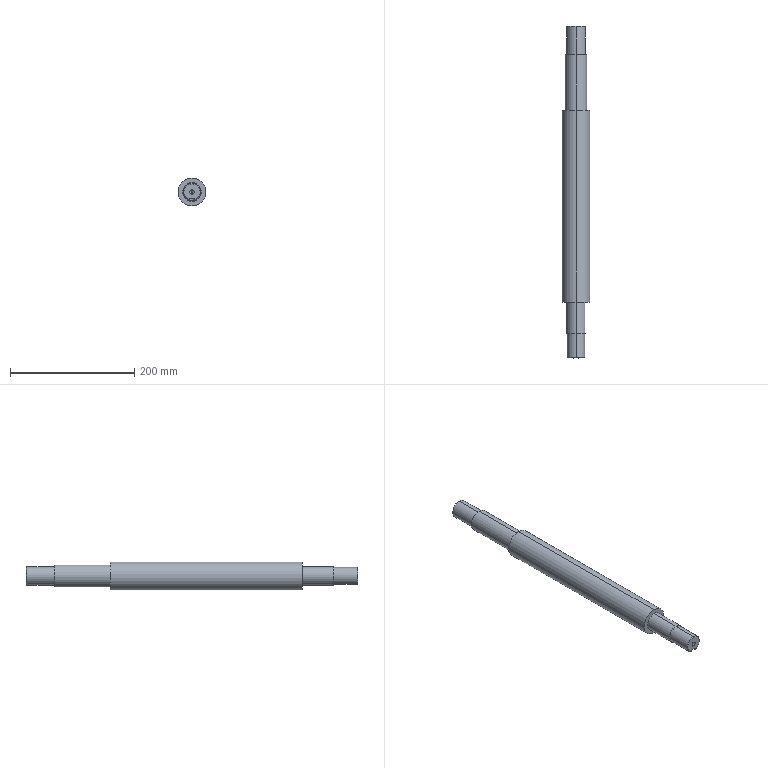Part | SolidWorks | features 3DProfileFeature 1, Chamfer 1, Cut 1, HoleWzd 1, Revolution 1 | 1 solid | 28 faces | box 45 x 535 x 45 mm | volume 668255 mm3 | cylinder 13 | plane 9 | cone 6 | commonest cylinder face diameters 30 x4 7 x2 28 x2 35 x2 45 x2 8 x1
STEP:
#1=CARTESIAN_POINT('',(0.,25.,3.5));
#2=VERTEX_POINT('',#1);
#3=CARTESIAN_POINT('',(0.,25.,-3.5));
#4=VERTEX_POINT('',#3);
#5=CARTESIAN_POINT('',(0.,25.,0.));
#6=DIRECTION('',(0.,-1.,0.));
#7=DIRECTION('',(0.,0.,-1.));
#8=AXIS2_PLACEMENT_3D('',#5,#6,#7);
#9=CIRCLE('',#8,3.5);
#10=EDGE_CURVE('',#2,#4,#9,.T.);
#11=ORIENTED_EDGE('',*,*,#10,.F.);
#12=CARTESIAN_POINT('',(0.,0.,3.5));
#13=VERTEX_POINT('',#12);
#14=CARTESIAN_POINT('',(0.,0.,3.5));
#15=DIRECTION('',(0.,-1.,0.));
#16=VECTOR('',#15,1000.);
#17=LINE('',#14,#16);
#18=EDGE_CURVE('',#2,#13,#17,.T.);
#19=ORIENTED_EDGE('',*,*,#18,.T.);
#20=CARTESIAN_POINT('',(0.,0.,-3.5));
#21=VERTEX_POINT('',#20);
#22=CARTESIAN_POINT('',(0.,0.,0.));
#23=DIRECTION('',(0.,-1.,0.));
#24=DIRECTION('',(0.,0.,-1.));
#25=AXIS2_PLACEMENT_3D('',#22,#23,#24);
#26=CIRCLE('',#25,3.5);
#27=EDGE_CURVE('',#13,#21,#26,.T.);
#28=ORIENTED_EDGE('',*,*,#27,.T.);
#29=CARTESIAN_POINT('',(0.,0.,-3.5));
#30=DIRECTION('',(0.,-1.,0.));
#31=VECTOR('',#30,1000.);
#32=LINE('',#29,#31);
#33=EDGE_CURVE('',#4,#21,#32,.T.);
#34=ORIENTED_EDGE('',*,*,#33,.F.);
#35=EDGE_LOOP('',(#11,#19,#28,#34));
#36=FACE_OUTER_BOUND('',#35,.T.);
#37=CARTESIAN_POINT('',(0.,0.,0.));
#38=DIRECTION('',(0.,-1.,0.));
#39=DIRECTION('',(0.,0.,-1.));
#40=AXIS2_PLACEMENT_3D('',#37,#38,#39);
#41=CYLINDRICAL_SURFACE('',#40,3.5);
#42=ADVANCED_FACE('',(#36),#41,.F.);
#43=CARTESIAN_POINT('',(0.,27.103,0.));
#44=VERTEX_POINT('',#43);
#45=CARTESIAN_POINT('',(0.,25.,-3.5));
#46=DIRECTION('',(0.,-0.515,-0.8572));
#47=VECTOR('',#46,1000.);
#48=LINE('',#45,#47);
#49=EDGE_CURVE('',#44,#4,#48,.T.);
#50=ORIENTED_EDGE('',*,*,#49,.F.);
#51=CARTESIAN_POINT('',(0.,25.,3.5));
#52=DIRECTION('',(0.,-0.515,0.8572));
#53=VECTOR('',#52,1000.);
#54=LINE('',#51,#53);
#55=EDGE_CURVE('',#44,#2,#54,.T.);
#56=ORIENTED_EDGE('',*,*,#55,.T.);
#57=ORIENTED_EDGE('',*,*,#10,.T.);
#58=EDGE_LOOP('',(#50,#56,#57));
#59=FACE_OUTER_BOUND('',#58,.T.);
#60=CARTESIAN_POINT('',(0.,25.,0.));
#61=DIRECTION('',(0.,-1.,0.));
#62=DIRECTION('',(0.,0.,-1.));
#63=AXIS2_PLACEMENT_3D('',#60,#61,#62);
#64=CONICAL_SURFACE('',#63,3.5,1.03);
#65=ADVANCED_FACE('',(#59),#64,.F.);
#66=CARTESIAN_POINT('',(0.,535.,14.));
#67=VERTEX_POINT('',#66);
#68=CARTESIAN_POINT('',(0.,535.,-14.));
#69=VERTEX_POINT('',#68);
#70=CARTESIAN_POINT('',(0.,535.,0.));
#71=DIRECTION('',(0.,1.,0.));
#72=DIRECTION('',(0.,0.,-1.));
#73=AXIS2_PLACEMENT_3D('',#70,#71,#72);
#74=CIRCLE('',#73,14.);
#75=EDGE_CURVE('',#67,#69,#74,.T.);
#76=ORIENTED_EDGE('',*,*,#75,.F.);
#77=CARTESIAN_POINT('',(0.,534.,15.));
#78=VERTEX_POINT('',#77);
#79=CARTESIAN_POINT('',(0.,535.,14.));
#80=DIRECTION('',(0.,-0.7071,0.7071));
#81=VECTOR('',#80,1000.);
#82=LINE('',#79,#81);
#83=EDGE_CURVE('',#67,#78,#82,.T.);
#84=ORIENTED_EDGE('',*,*,#83,.T.);
#85=CARTESIAN_POINT('',(0.,534.,-15.));
#86=VERTEX_POINT('',#85);
#87=CARTESIAN_POINT('',(0.,534.,0.));
#88=DIRECTION('',(0.,-1.,0.));
#89=DIRECTION('',(0.,0.,-1.));
#90=AXIS2_PLACEMENT_3D('',#87,#88,#89);
#91=CIRCLE('',#90,15.);
#92=EDGE_CURVE('',#86,#78,#91,.T.);
#93=ORIENTED_EDGE('',*,*,#92,.F.);
#94=CARTESIAN_POINT('',(0.,535.,-14.));
#95=DIRECTION('',(0.,-0.7071,-0.7071));
#96=VECTOR('',#95,1000.);
#97=LINE('',#94,#96);
#98=EDGE_CURVE('',#69,#86,#97,.T.);
#99=ORIENTED_EDGE('',*,*,#98,.F.);
#100=EDGE_LOOP('',(#76,#84,#93,#99));
#101=FACE_OUTER_BOUND('',#100,.T.);
#102=CARTESIAN_POINT('',(0.,535.,0.));
#103=DIRECTION('',(0.,-1.,0.));
#104=DIRECTION('',(0.,0.,-1.));
#105=AXIS2_PLACEMENT_3D('',#102,#103,#104);
#106=CONICAL_SURFACE('',#105,14.,0.7854);
#107=ADVANCED_FACE('',(#101),#106,.T.);
#108=CARTESIAN_POINT('',(0.,0.,13.));
#109=VERTEX_POINT('',#108);
#110=CARTESIAN_POINT('',(-4.,0.,-12.369));
#111=VERTEX_POINT('',#110);
#112=CARTESIAN_POINT('',(0.,0.,0.));
#113=DIRECTION('',(0.,-1.,0.));
#114=DIRECTION('',(0.,0.,1.));
#115=AXIS2_PLACEMENT_3D('',#112,#113,#114);
#116=CIRCLE('',#115,13.);
#117=EDGE_CURVE('',#109,#111,#116,.T.);
#118=ORIENTED_EDGE('',*,*,#117,.F.);
#119=CARTESIAN_POINT('',(0.,1.,14.));
#120=VERTEX_POINT('',#119);
#121=CARTESIAN_POINT('',(0.,1.,14.));
#122=DIRECTION('',(0.,0.7071,0.7071));
#123=VECTOR('',#122,1000.);
#124=LINE('',#121,#123);
#125=EDGE_CURVE('',#109,#120,#124,.T.);
#126=ORIENTED_EDGE('',*,*,#125,.T.);
#127=CARTESIAN_POINT('',(-4.,1.,-13.416));
#128=VERTEX_POINT('',#127);
#129=CARTESIAN_POINT('',(0.,1.,0.));
#130=DIRECTION('',(0.,1.,0.));
#131=DIRECTION('',(0.,0.,1.));
#132=AXIS2_PLACEMENT_3D('',#129,#130,#131);
#133=CIRCLE('',#132,14.);
#134=EDGE_CURVE('',#128,#120,#133,.T.);
#135=ORIENTED_EDGE('',*,*,#134,.F.);
#136=CARTESIAN_POINT('',(-4.,0.,-12.369));
#137=CARTESIAN_POINT('',(-4.,0.3327,-12.719));
#138=CARTESIAN_POINT('',(-4.,0.6661,-13.068));
#139=CARTESIAN_POINT('',(-4.,1.,-13.416));
#140=B_SPLINE_CURVE_WITH_KNOTS('',3,(#136,#137,#138,#139),.UNSPECIFIED.,.F.,.F.,(4,4),(0.006639,0.008087),.UNSPECIFIED.);
#141=EDGE_CURVE('',#111,#128,#140,.T.);
#142=ORIENTED_EDGE('',*,*,#141,.F.);
#143=EDGE_LOOP('',(#118,#126,#135,#142));
#144=FACE_OUTER_BOUND('',#143,.T.);
#145=CARTESIAN_POINT('',(0.,1.,0.));
#146=DIRECTION('',(0.,1.,0.));
#147=DIRECTION('',(0.,0.,1.));
#148=AXIS2_PLACEMENT_3D('',#145,#146,#147);
#149=CONICAL_SURFACE('',#148,14.,0.7854);
#150=ADVANCED_FACE('',(#144),#149,.T.);
#151=CARTESIAN_POINT('',(0.,489.,15.));
#152=VERTEX_POINT('',#151);
#153=CARTESIAN_POINT('',(0.,489.,-15.));
#154=VERTEX_POINT('',#153);
#155=CARTESIAN_POINT('',(0.,489.,0.));
#156=DIRECTION('',(0.,1.,0.));
#157=DIRECTION('',(0.,0.,1.));
#158=AXIS2_PLACEMENT_3D('',#155,#156,#157);
#159=CIRCLE('',#158,15.);
#160=EDGE_CURVE('',#152,#154,#159,.T.);
#161=ORIENTED_EDGE('',*,*,#160,.T.);
#162=CARTESIAN_POINT('',(0.,535.,-15.));
#163=DIRECTION('',(0.,1.,0.));
#164=VECTOR('',#163,1000.);
#165=LINE('',#162,#164);
#166=EDGE_CURVE('',#154,#86,#165,.T.);
#167=ORIENTED_EDGE('',*,*,#166,.T.);
#168=ORIENTED_EDGE('',*,*,#92,.T.);
#169=CARTESIAN_POINT('',(0.,535.,15.));
#170=DIRECTION('',(0.,1.,0.));
#171=VECTOR('',#170,1000.);
#172=LINE('',#169,#171);
#173=EDGE_CURVE('',#152,#78,#172,.T.);
#174=ORIENTED_EDGE('',*,*,#173,.F.);
#175=EDGE_LOOP('',(#161,#167,#168,#174));
#176=FACE_OUTER_BOUND('',#175,.T.);
#177=CARTESIAN_POINT('',(0.,535.,0.));
#178=DIRECTION('',(0.,1.,0.));
#179=DIRECTION('',(0.,0.,1.));
#180=AXIS2_PLACEMENT_3D('',#177,#178,#179);
#181=CYLINDRICAL_SURFACE('',#180,15.);
#182=ADVANCED_FACE('',(#176),#181,.T.);
#183=CARTESIAN_POINT('',(0.,399.,17.5));
#184=VERTEX_POINT('',#183);
#185=CARTESIAN_POINT('',(0.,399.,-17.5));
#186=VERTEX_POINT('',#185);
#187=CARTESIAN_POINT('',(0.,399.,0.));
#188=DIRECTION('',(0.,1.,0.));
#189=DIRECTION('',(0.,0.,1.));
#190=AXIS2_PLACEMENT_3D('',#187,#188,#189);
#191=CIRCLE('',#190,17.5);
#192=EDGE_CURVE('',#184,#186,#191,.T.);
#193=ORIENTED_EDGE('',*,*,#192,.T.);
#194=CARTESIAN_POINT('',(0.,489.,-17.5));
#195=VERTEX_POINT('',#194);
#196=CARTESIAN_POINT('',(0.,535.,-17.5));
#197=DIRECTION('',(0.,1.,0.));
#198=VECTOR('',#197,1000.);
#199=LINE('',#196,#198);
#200=EDGE_CURVE('',#186,#195,#199,.T.);
#201=ORIENTED_EDGE('',*,*,#200,.T.);
#202=CARTESIAN_POINT('',(0.,489.,17.5));
#203=VERTEX_POINT('',#202);
#204=CARTESIAN_POINT('',(0.,489.,0.));
#205=DIRECTION('',(0.,1.,0.));
#206=DIRECTION('',(0.,0.,1.));
#207=AXIS2_PLACEMENT_3D('',#204,#205,#206);
#208=CIRCLE('',#207,17.5);
#209=EDGE_CURVE('',#203,#195,#208,.T.);
#210=ORIENTED_EDGE('',*,*,#209,.F.);
#211=CARTESIAN_POINT('',(0.,535.,17.5));
#212=DIRECTION('',(0.,1.,0.));
#213=VECTOR('',#212,1000.);
#214=LINE('',#211,#213);
#215=EDGE_CURVE('',#184,#203,#214,.T.);
#216=ORIENTED_EDGE('',*,*,#215,.F.);
#217=EDGE_LOOP('',(#193,#201,#210,#216));
#218=FACE_OUTER_BOUND('',#217,.T.);
#219=CARTESIAN_POINT('',(0.,535.,0.));
#220=DIRECTION('',(0.,1.,0.));
#221=DIRECTION('',(0.,0.,1.));
#222=AXIS2_PLACEMENT_3D('',#219,#220,#221);
#223=CYLINDRICAL_SURFACE('',#222,17.5);
#224=ADVANCED_FACE('',(#218),#223,.T.);
#225=CARTESIAN_POINT('',(0.,90.,22.5));
#226=VERTEX_POINT('',#225);
#227=CARTESIAN_POINT('',(0.,90.,-22.5));
#228=VERTEX_POINT('',#227);
#229=CARTESIAN_POINT('',(0.,90.,0.));
#230=DIRECTION('',(0.,1.,0.));
#231=DIRECTION('',(0.,0.,1.));
#232=AXIS2_PLACEMENT_3D('',#229,#230,#231);
#233=CIRCLE('',#232,22.5);
#234=EDGE_CURVE('',#226,#228,#233,.T.);
#235=ORIENTED_EDGE('',*,*,#234,.T.);
#236=CARTESIAN_POINT('',(0.,399.,-22.5));
#237=VERTEX_POINT('',#236);
#238=CARTESIAN_POINT('',(0.,535.,-22.5));
#239=DIRECTION('',(0.,1.,0.));
#240=VECTOR('',#239,1000.);
#241=LINE('',#238,#240);
#242=EDGE_CURVE('',#228,#237,#241,.T.);
#243=ORIENTED_EDGE('',*,*,#242,.T.);
#244=CARTESIAN_POINT('',(0.,399.,22.5));
#245=VERTEX_POINT('',#244);
#246=CARTESIAN_POINT('',(0.,399.,0.));
#247=DIRECTION('',(0.,1.,0.));
#248=DIRECTION('',(0.,0.,1.));
#249=AXIS2_PLACEMENT_3D('',#246,#247,#248);
#250=CIRCLE('',#249,22.5);
#251=EDGE_CURVE('',#245,#237,#250,.T.);
#252=ORIENTED_EDGE('',*,*,#251,.F.);
#253=CARTESIAN_POINT('',(0.,535.,22.5));
#254=DIRECTION('',(0.,1.,0.));
#255=VECTOR('',#254,1000.);
#256=LINE('',#253,#255);
#257=EDGE_CURVE('',#226,#245,#256,.T.);
#258=ORIENTED_EDGE('',*,*,#257,.F.);
#259=EDGE_LOOP('',(#235,#243,#252,#258));
#260=FACE_OUTER_BOUND('',#259,.T.);
#261=CARTESIAN_POINT('',(0.,535.,0.));
#262=DIRECTION('',(0.,1.,0.));
#263=DIRECTION('',(0.,0.,1.));
#264=AXIS2_PLACEMENT_3D('',#261,#262,#263);
#265=CYLINDRICAL_SURFACE('',#264,22.5);
#266=ADVANCED_FACE('',(#260),#265,.T.);
#267=CARTESIAN_POINT('',(0.,40.,15.));
#268=VERTEX_POINT('',#267);
#269=CARTESIAN_POINT('',(0.,40.,-15.));
#270=VERTEX_POINT('',#269);
#271=CARTESIAN_POINT('',(0.,40.,0.));
#272=DIRECTION('',(0.,1.,0.));
#273=DIRECTION('',(0.,0.,1.));
#274=AXIS2_PLACEMENT_3D('',#271,#272,#273);
#275=CIRCLE('',#274,15.);
#276=EDGE_CURVE('',#268,#270,#275,.T.);
#277=ORIENTED_EDGE('',*,*,#276,.T.);
#278=CARTESIAN_POINT('',(0.,90.,-15.));
#279=VERTEX_POINT('',#278);
#280=CARTESIAN_POINT('',(0.,535.,-15.));
#281=DIRECTION('',(0.,1.,0.));
#282=VECTOR('',#281,1000.);
#283=LINE('',#280,#282);
#284=EDGE_CURVE('',#270,#279,#283,.T.);
#285=ORIENTED_EDGE('',*,*,#284,.T.);
#286=CARTESIAN_POINT('',(0.,90.,15.));
#287=VERTEX_POINT('',#286);
#288=CARTESIAN_POINT('',(0.,90.,0.));
#289=DIRECTION('',(0.,1.,0.));
#290=DIRECTION('',(0.,0.,1.));
#291=AXIS2_PLACEMENT_3D('',#288,#289,#290);
#292=CIRCLE('',#291,15.);
#293=EDGE_CURVE('',#287,#279,#292,.T.);
#294=ORIENTED_EDGE('',*,*,#293,.F.);
#295=CARTESIAN_POINT('',(0.,535.,15.));
#296=DIRECTION('',(0.,1.,0.));
#297=VECTOR('',#296,1000.);
#298=LINE('',#295,#297);
#299=EDGE_CURVE('',#268,#287,#298,.T.);
#300=ORIENTED_EDGE('',*,*,#299,.F.);
#301=EDGE_LOOP('',(#277,#285,#294,#300));
#302=FACE_OUTER_BOUND('',#301,.T.);
#303=CARTESIAN_POINT('',(0.,535.,0.));
#304=DIRECTION('',(0.,1.,0.));
#305=DIRECTION('',(0.,0.,1.));
#306=AXIS2_PLACEMENT_3D('',#303,#304,#305);
#307=CYLINDRICAL_SURFACE('',#306,15.);
#308=ADVANCED_FACE('',(#302),#307,.T.);
#309=ORIENTED_EDGE('',*,*,#134,.T.);
#310=CARTESIAN_POINT('',(0.,40.,14.));
#311=VERTEX_POINT('',#310);
#312=CARTESIAN_POINT('',(0.,535.,14.));
#313=DIRECTION('',(0.,1.,0.));
#314=VECTOR('',#313,1000.);
#315=LINE('',#312,#314);
#316=EDGE_CURVE('',#120,#311,#315,.T.);
#317=ORIENTED_EDGE('',*,*,#316,.T.);
#318=CARTESIAN_POINT('',(0.,40.,-14.));
#319=VERTEX_POINT('',#318);
#320=CARTESIAN_POINT('',(0.,40.,0.));
#321=DIRECTION('',(0.,1.,0.));
#322=DIRECTION('',(0.,0.,1.));
#323=AXIS2_PLACEMENT_3D('',#320,#321,#322);
#324=CIRCLE('',#323,14.);
#325=EDGE_CURVE('',#319,#311,#324,.T.);
#326=ORIENTED_EDGE('',*,*,#325,.F.);
#327=CARTESIAN_POINT('',(-4.,36.,-13.416));
#328=VERTEX_POINT('',#327);
#329=CARTESIAN_POINT('',(0.,40.,-14.));
#330=CARTESIAN_POINT('',(-0.2622,40.,-14.));
#331=CARTESIAN_POINT('',(-0.5286,39.974,-13.992));
#332=CARTESIAN_POINT('',(-1.042,39.871,-13.964));
#333=CARTESIAN_POINT('',(-1.292,39.795,-13.942));
#334=CARTESIAN_POINT('',(-1.778,39.593,-13.889));
#335=CARTESIAN_POINT('',(-2.009,39.468,-13.857));
#336=CARTESIAN_POINT('',(-2.441,39.18,-13.787));
#337=CARTESIAN_POINT('',(-2.644,39.013,-13.749));
#338=CARTESIAN_POINT('',(-3.013,38.643,-13.673));
#339=CARTESIAN_POINT('',(-3.178,38.443,-13.635));
#340=CARTESIAN_POINT('',(-3.467,38.011,-13.565));
#341=CARTESIAN_POINT('',(-3.593,37.778,-13.532));
#342=CARTESIAN_POINT('',(-3.793,37.296,-13.477));
#343=CARTESIAN_POINT('',(-3.87,37.047,-13.455));
#344=CARTESIAN_POINT('',(-3.973,36.531,-13.424));
#345=CARTESIAN_POINT('',(-4.,36.266,-13.416));
#346=CARTESIAN_POINT('',(-4.,36.,-13.416));
#347=B_SPLINE_CURVE_WITH_KNOTS('',3,(#329,#330,#331,#332,#333,#334,#335,#336,#337,#338,#339,#340,#341,#342,#343,#344,#345,#346),.UNSPECIFIED.,.F.,.F.,(4,2,2,2,2,2,2,2,4),(0.006287,0.007072,0.007857,0.008642,0.009427,0.01021,0.011,0.01178,0.01257),.UNSPECIFIED.);
#348=EDGE_CURVE('',#319,#328,#347,.T.);
#349=ORIENTED_EDGE('',*,*,#348,.T.);
#350=CARTESIAN_POINT('',(-4.,535.,-13.416));
#351=DIRECTION('',(0.,-1.,0.));
#352=VECTOR('',#351,1000.);
#353=LINE('',#350,#352);
#354=EDGE_CURVE('',#328,#128,#353,.T.);
#355=ORIENTED_EDGE('',*,*,#354,.T.);
#356=EDGE_LOOP('',(#309,#317,#326,#349,#355));
#357=FACE_OUTER_BOUND('',#356,.T.);
#358=CARTESIAN_POINT('',(0.,535.,0.));
#359=DIRECTION('',(0.,1.,0.));
#360=DIRECTION('',(0.,0.,1.));
#361=AXIS2_PLACEMENT_3D('',#358,#359,#360);
#362=CYLINDRICAL_SURFACE('',#361,14.);
#363=ADVANCED_FACE('',(#357),#362,.T.);
#364=CARTESIAN_POINT('',(0.,0.,0.));
#365=DIRECTION('',(0.,-1.,0.));
#366=DIRECTION('',(0.,0.,-1.));
#367=AXIS2_PLACEMENT_3D('',#364,#365,#366);
#368=CIRCLE('',#367,3.5);
#369=EDGE_CURVE('',#21,#13,#368,.T.);
#370=ORIENTED_EDGE('',*,*,#369,.F.);
#371=ORIENTED_EDGE('',*,*,#27,.F.);
#372=EDGE_LOOP('',(#370,#371));
#373=FACE_BOUND('',#372,.T.);
#374=CARTESIAN_POINT('',(-4.,0.,-10.));
#375=VERTEX_POINT('',#374);
#376=CARTESIAN_POINT('',(4.,0.,-10.));
#377=VERTEX_POINT('',#376);
#378=CARTESIAN_POINT('',(0.,0.,-10.));
#379=DIRECTION('',(1.,0.,0.));
#380=VECTOR('',#379,1000.);
#381=LINE('',#378,#380);
#382=EDGE_CURVE('',#375,#377,#381,.T.);
#383=ORIENTED_EDGE('',*,*,#382,.T.);
#384=CARTESIAN_POINT('',(4.,0.,-12.369));
#385=VERTEX_POINT('',#384);
#386=CARTESIAN_POINT('',(4.,0.,-15.));
#387=DIRECTION('',(0.,0.,1.));
#388=VECTOR('',#387,1000.);
#389=LINE('',#386,#388);
#390=EDGE_CURVE('',#385,#377,#389,.T.);
#391=ORIENTED_EDGE('',*,*,#390,.F.);
#392=CARTESIAN_POINT('',(0.,0.,0.));
#393=DIRECTION('',(0.,-1.,0.));
#394=DIRECTION('',(0.,0.,1.));
#395=AXIS2_PLACEMENT_3D('',#392,#393,#394);
#396=CIRCLE('',#395,13.);
#397=EDGE_CURVE('',#385,#109,#396,.T.);
#398=ORIENTED_EDGE('',*,*,#397,.T.);
#399=ORIENTED_EDGE('',*,*,#117,.T.);
#400=CARTESIAN_POINT('',(-4.,0.,-15.));
#401=DIRECTION('',(0.,0.,1.));
#402=VECTOR('',#401,1000.);
#403=LINE('',#400,#402);
#404=EDGE_CURVE('',#111,#375,#403,.T.);
#405=ORIENTED_EDGE('',*,*,#404,.T.);
#406=EDGE_LOOP('',(#383,#391,#398,#399,#405));
#407=FACE_OUTER_BOUND('',#406,.T.);
#408=CARTESIAN_POINT('',(0.,0.,0.));
#409=DIRECTION('',(0.,1.,0.));
#410=DIRECTION('',(0.,0.,1.));
#411=AXIS2_PLACEMENT_3D('',#408,#409,#410);
#412=PLANE('',#411);
#413=ADVANCED_FACE('',(#373,#407),#412,.F.);
#414=ORIENTED_EDGE('',*,*,#316,.F.);
#415=CARTESIAN_POINT('',(4.,1.,-13.416));
#416=VERTEX_POINT('',#415);
#417=CARTESIAN_POINT('',(0.,1.,0.));
#418=DIRECTION('',(0.,1.,0.));
#419=DIRECTION('',(0.,0.,1.));
#420=AXIS2_PLACEMENT_3D('',#417,#418,#419);
#421=CIRCLE('',#420,14.);
#422=EDGE_CURVE('',#120,#416,#421,.T.);
#423=ORIENTED_EDGE('',*,*,#422,.T.);
#424=CARTESIAN_POINT('',(4.,36.,-13.416));
#425=VERTEX_POINT('',#424);
#426=CARTESIAN_POINT('',(4.,535.,-13.416));
#427=DIRECTION('',(0.,1.,0.));
#428=VECTOR('',#427,1000.);
#429=LINE('',#426,#428);
#430=EDGE_CURVE('',#416,#425,#429,.T.);
#431=ORIENTED_EDGE('',*,*,#430,.T.);
#432=CARTESIAN_POINT('',(4.,36.,-13.416));
#433=CARTESIAN_POINT('',(4.,36.266,-13.416));
#434=CARTESIAN_POINT('',(3.974,36.527,-13.424));
#435=CARTESIAN_POINT('',(3.871,37.04,-13.454));
#436=CARTESIAN_POINT('',(3.794,37.295,-13.477));
#437=CARTESIAN_POINT('',(3.592,37.779,-13.532));
#438=CARTESIAN_POINT('',(3.469,38.008,-13.564));
#439=CARTESIAN_POINT('',(3.179,38.442,-13.635));
#440=CARTESIAN_POINT('',(3.011,38.646,-13.674));
#441=CARTESIAN_POINT('',(2.644,39.013,-13.749));
#442=CARTESIAN_POINT('',(2.443,39.178,-13.787));
#443=CARTESIAN_POINT('',(2.006,39.471,-13.857));
#444=CARTESIAN_POINT('',(1.775,39.594,-13.889));
#445=CARTESIAN_POINT('',(1.294,39.794,-13.942));
#446=CARTESIAN_POINT('',(1.04,39.871,-13.964));
#447=CARTESIAN_POINT('',(0.5231,39.974,-13.993));
#448=CARTESIAN_POINT('',(0.2626,40.,-14.));
#449=CARTESIAN_POINT('',(0.,40.,-14.));
#450=B_SPLINE_CURVE_WITH_KNOTS('',3,(#432,#433,#434,#435,#436,#437,#438,#439,#440,#441,#442,#443,#444,#445,#446,#447,#448,#449),.UNSPECIFIED.,.F.,.F.,(4,2,2,2,2,2,2,2,4),(0.,0.0007859,0.001572,0.002358,0.003144,0.00393,0.004716,0.005502,0.006287),.UNSPECIFIED.);
#451=EDGE_CURVE('',#425,#319,#450,.T.);
#452=ORIENTED_EDGE('',*,*,#451,.T.);
#453=CARTESIAN_POINT('',(0.,40.,0.));
#454=DIRECTION('',(0.,1.,0.));
#455=DIRECTION('',(0.,0.,1.));
#456=AXIS2_PLACEMENT_3D('',#453,#454,#455);
#457=CIRCLE('',#456,14.);
#458=EDGE_CURVE('',#311,#319,#457,.T.);
#459=ORIENTED_EDGE('',*,*,#458,.F.);
#460=EDGE_LOOP('',(#414,#423,#431,#452,#459));
#461=FACE_OUTER_BOUND('',#460,.T.);
#462=CARTESIAN_POINT('',(0.,535.,0.));
#463=DIRECTION('',(0.,1.,0.));
#464=DIRECTION('',(0.,0.,1.));
#465=AXIS2_PLACEMENT_3D('',#462,#463,#464);
#466=CYLINDRICAL_SURFACE('',#465,14.);
#467=ADVANCED_FACE('',(#461),#466,.T.);
#468=ORIENTED_EDGE('',*,*,#325,.T.);
#469=ORIENTED_EDGE('',*,*,#458,.T.);
#470=EDGE_LOOP('',(#468,#469));
#471=FACE_BOUND('',#470,.T.);
#472=ORIENTED_EDGE('',*,*,#276,.F.);
#473=CARTESIAN_POINT('',(0.,40.,0.));
#474=DIRECTION('',(0.,1.,0.));
#475=DIRECTION('',(0.,0.,1.));
#476=AXIS2_PLACEMENT_3D('',#473,#474,#475);
#477=CIRCLE('',#476,15.);
#478=EDGE_CURVE('',#270,#268,#477,.T.);
#479=ORIENTED_EDGE('',*,*,#478,.F.);
#480=EDGE_LOOP('',(#472,#479));
#481=FACE_OUTER_BOUND('',#480,.T.);
#482=CARTESIAN_POINT('',(14.,40.,0.));
#483=DIRECTION('',(0.,1.,0.));
#484=DIRECTION('',(0.,0.,1.));
#485=AXIS2_PLACEMENT_3D('',#482,#483,#484);
#486=PLANE('',#485);
#487=ADVANCED_FACE('',(#471,#481),#486,.F.);
#488=ORIENTED_EDGE('',*,*,#284,.F.);
#489=ORIENTED_EDGE('',*,*,#478,.T.);
#490=ORIENTED_EDGE('',*,*,#299,.T.);
#491=CARTESIAN_POINT('',(0.,90.,0.));
#492=DIRECTION('',(0.,1.,0.));
#493=DIRECTION('',(0.,0.,1.));
#494=AXIS2_PLACEMENT_3D('',#491,#492,#493);
#495=CIRCLE('',#494,15.);
#496=EDGE_CURVE('',#279,#287,#495,.T.);
#497=ORIENTED_EDGE('',*,*,#496,.F.);
#498=EDGE_LOOP('',(#488,#489,#490,#497));
#499=FACE_OUTER_BOUND('',#498,.T.);
#500=CARTESIAN_POINT('',(0.,535.,0.));
#501=DIRECTION('',(0.,1.,0.));
#502=DIRECTION('',(0.,0.,1.));
#503=AXIS2_PLACEMENT_3D('',#500,#501,#502);
#504=CYLINDRICAL_SURFACE('',#503,15.);
#505=ADVANCED_FACE('',(#499),#504,.T.);
#506=ORIENTED_EDGE('',*,*,#234,.F.);
#507=CARTESIAN_POINT('',(0.,90.,0.));
#508=DIRECTION('',(0.,1.,0.));
#509=DIRECTION('',(0.,0.,1.));
#510=AXIS2_PLACEMENT_3D('',#507,#508,#509);
#511=CIRCLE('',#510,22.5);
#512=EDGE_CURVE('',#228,#226,#511,.T.);
#513=ORIENTED_EDGE('',*,*,#512,.F.);
#514=EDGE_LOOP('',(#506,#513));
#515=FACE_OUTER_BOUND('',#514,.T.);
#516=ORIENTED_EDGE('',*,*,#293,.T.);
#517=ORIENTED_EDGE('',*,*,#496,.T.);
#518=EDGE_LOOP('',(#516,#517));
#519=FACE_BOUND('',#518,.T.);
#520=CARTESIAN_POINT('',(15.,90.,0.));
#521=DIRECTION('',(0.,1.,0.));
#522=DIRECTION('',(0.,0.,1.));
#523=AXIS2_PLACEMENT_3D('',#520,#521,#522);
#524=PLANE('',#523);
#525=ADVANCED_FACE('',(#515,#519),#524,.F.);
#526=ORIENTED_EDGE('',*,*,#242,.F.);
#527=ORIENTED_EDGE('',*,*,#512,.T.);
#528=ORIENTED_EDGE('',*,*,#257,.T.);
#529=CARTESIAN_POINT('',(0.,399.,0.));
#530=DIRECTION('',(0.,1.,0.));
#531=DIRECTION('',(0.,0.,1.));
#532=AXIS2_PLACEMENT_3D('',#529,#530,#531);
#533=CIRCLE('',#532,22.5);
#534=EDGE_CURVE('',#237,#245,#533,.T.);
#535=ORIENTED_EDGE('',*,*,#534,.F.);
#536=EDGE_LOOP('',(#526,#527,#528,#535));
#537=FACE_OUTER_BOUND('',#536,.T.);
#538=CARTESIAN_POINT('',(0.,535.,0.));
#539=DIRECTION('',(0.,1.,0.));
#540=DIRECTION('',(0.,0.,1.));
#541=AXIS2_PLACEMENT_3D('',#538,#539,#540);
#542=CYLINDRICAL_SURFACE('',#541,22.5);
#543=ADVANCED_FACE('',(#537),#542,.T.);
#544=ORIENTED_EDGE('',*,*,#192,.F.);
#545=CARTESIAN_POINT('',(0.,399.,0.));
#546=DIRECTION('',(0.,1.,0.));
#547=DIRECTION('',(0.,0.,1.));
#548=AXIS2_PLACEMENT_3D('',#545,#546,#547);
#549=CIRCLE('',#548,17.5);
#550=EDGE_CURVE('',#186,#184,#549,.T.);
#551=ORIENTED_EDGE('',*,*,#550,.F.);
#552=EDGE_LOOP('',(#544,#551));
#553=FACE_BOUND('',#552,.T.);
#554=ORIENTED_EDGE('',*,*,#251,.T.);
#555=ORIENTED_EDGE('',*,*,#534,.T.);
#556=EDGE_LOOP('',(#554,#555));
#557=FACE_OUTER_BOUND('',#556,.T.);
#558=CARTESIAN_POINT('',(22.5,399.,0.));
#559=DIRECTION('',(0.,-1.,0.));
#560=DIRECTION('',(0.,0.,-1.));
#561=AXIS2_PLACEMENT_3D('',#558,#559,#560);
#562=PLANE('',#561);
#563=ADVANCED_FACE('',(#553,#557),#562,.F.);
#564=ORIENTED_EDGE('',*,*,#200,.F.);
#565=ORIENTED_EDGE('',*,*,#550,.T.);
#566=ORIENTED_EDGE('',*,*,#215,.T.);
#567=CARTESIAN_POINT('',(0.,489.,0.));
#568=DIRECTION('',(0.,1.,0.));
#569=DIRECTION('',(0.,0.,1.));
#570=AXIS2_PLACEMENT_3D('',#567,#568,#569);
#571=CIRCLE('',#570,17.5);
#572=EDGE_CURVE('',#195,#203,#571,.T.);
#573=ORIENTED_EDGE('',*,*,#572,.F.);
#574=EDGE_LOOP('',(#564,#565,#566,#573));
#575=FACE_OUTER_BOUND('',#574,.T.);
#576=CARTESIAN_POINT('',(0.,535.,0.));
#577=DIRECTION('',(0.,1.,0.));
#578=DIRECTION('',(0.,0.,1.));
#579=AXIS2_PLACEMENT_3D('',#576,#577,#578);
#580=CYLINDRICAL_SURFACE('',#579,17.5);
#581=ADVANCED_FACE('',(#575),#580,.T.);
#582=ORIENTED_EDGE('',*,*,#160,.F.);
#583=CARTESIAN_POINT('',(0.,489.,0.));
#584=DIRECTION('',(0.,1.,0.));
#585=DIRECTION('',(0.,0.,1.));
#586=AXIS2_PLACEMENT_3D('',#583,#584,#585);
#587=CIRCLE('',#586,15.);
#588=EDGE_CURVE('',#154,#152,#587,.T.);
#589=ORIENTED_EDGE('',*,*,#588,.F.);
#590=EDGE_LOOP('',(#582,#589));
#591=FACE_BOUND('',#590,.T.);
#592=ORIENTED_EDGE('',*,*,#209,.T.);
#593=ORIENTED_EDGE('',*,*,#572,.T.);
#594=EDGE_LOOP('',(#592,#593));
#595=FACE_OUTER_BOUND('',#594,.T.);
#596=CARTESIAN_POINT('',(17.5,489.,0.));
#597=DIRECTION('',(0.,-1.,0.));
#598=DIRECTION('',(0.,0.,-1.));
#599=AXIS2_PLACEMENT_3D('',#596,#597,#598);
#600=PLANE('',#599);
#601=ADVANCED_FACE('',(#591,#595),#600,.F.);
#602=ORIENTED_EDGE('',*,*,#166,.F.);
#603=ORIENTED_EDGE('',*,*,#588,.T.);
#604=ORIENTED_EDGE('',*,*,#173,.T.);
#605=CARTESIAN_POINT('',(0.,534.,0.));
#606=DIRECTION('',(0.,-1.,0.));
#607=DIRECTION('',(0.,0.,-1.));
#608=AXIS2_PLACEMENT_3D('',#605,#606,#607);
#609=CIRCLE('',#608,15.);
#610=EDGE_CURVE('',#78,#86,#609,.T.);
#611=ORIENTED_EDGE('',*,*,#610,.T.);
#612=EDGE_LOOP('',(#602,#603,#604,#611));
#613=FACE_OUTER_BOUND('',#612,.T.);
#614=CARTESIAN_POINT('',(0.,535.,0.));
#615=DIRECTION('',(0.,1.,0.));
#616=DIRECTION('',(0.,0.,1.));
#617=AXIS2_PLACEMENT_3D('',#614,#615,#616);
#618=CYLINDRICAL_SURFACE('',#617,15.);
#619=ADVANCED_FACE('',(#613),#618,.T.);
#620=CARTESIAN_POINT('',(0.,535.,0.));
#621=DIRECTION('',(0.,1.,0.));
#622=DIRECTION('',(0.,0.,-1.));
#623=AXIS2_PLACEMENT_3D('',#620,#621,#622);
#624=CIRCLE('',#623,14.);
#625=EDGE_CURVE('',#69,#67,#624,.T.);
#626=ORIENTED_EDGE('',*,*,#625,.T.);
#627=ORIENTED_EDGE('',*,*,#75,.T.);
#628=EDGE_LOOP('',(#626,#627));
#629=FACE_OUTER_BOUND('',#628,.T.);
#630=CARTESIAN_POINT('',(15.,535.,0.));
#631=DIRECTION('',(0.,-1.,0.));
#632=DIRECTION('',(0.,0.,-1.));
#633=AXIS2_PLACEMENT_3D('',#630,#631,#632);
#634=PLANE('',#633);
#635=ADVANCED_FACE('',(#629),#634,.F.);
#636=ORIENTED_EDGE('',*,*,#125,.F.);
#637=ORIENTED_EDGE('',*,*,#397,.F.);
#638=CARTESIAN_POINT('',(4.,1.,-13.416));
#639=CARTESIAN_POINT('',(4.,0.6661,-13.068));
#640=CARTESIAN_POINT('',(4.,0.3327,-12.719));
#641=CARTESIAN_POINT('',(4.,0.,-12.369));
#642=B_SPLINE_CURVE_WITH_KNOTS('',3,(#638,#639,#640,#641),.UNSPECIFIED.,.F.,.F.,(4,4),(0.007514,0.008962),.UNSPECIFIED.);
#643=EDGE_CURVE('',#416,#385,#642,.T.);
#644=ORIENTED_EDGE('',*,*,#643,.F.);
#645=ORIENTED_EDGE('',*,*,#422,.F.);
#646=EDGE_LOOP('',(#636,#637,#644,#645));
#647=FACE_OUTER_BOUND('',#646,.T.);
#648=CARTESIAN_POINT('',(0.,1.,0.));
#649=DIRECTION('',(0.,1.,0.));
#650=DIRECTION('',(0.,0.,1.));
#651=AXIS2_PLACEMENT_3D('',#648,#649,#650);
#652=CONICAL_SURFACE('',#651,14.,0.7854);
#653=ADVANCED_FACE('',(#647),#652,.T.);
#654=ORIENTED_EDGE('',*,*,#83,.F.);
#655=ORIENTED_EDGE('',*,*,#625,.F.);
#656=ORIENTED_EDGE('',*,*,#98,.T.);
#657=ORIENTED_EDGE('',*,*,#610,.F.);
#658=EDGE_LOOP('',(#654,#655,#656,#657));
#659=FACE_OUTER_BOUND('',#658,.T.);
#660=CARTESIAN_POINT('',(0.,535.,0.));
#661=DIRECTION('',(0.,-1.,0.));
#662=DIRECTION('',(0.,0.,-1.));
#663=AXIS2_PLACEMENT_3D('',#660,#661,#662);
#664=CONICAL_SURFACE('',#663,14.,0.7854);
#665=ADVANCED_FACE('',(#659),#664,.T.);
#666=CARTESIAN_POINT('',(-4.,36.,-10.));
#667=VERTEX_POINT('',#666);
#668=CARTESIAN_POINT('',(-4.,36.,-10.));
#669=DIRECTION('',(0.,-1.,0.));
#670=VECTOR('',#669,1000.);
#671=LINE('',#668,#670);
#672=EDGE_CURVE('',#667,#375,#671,.T.);
#673=ORIENTED_EDGE('',*,*,#672,.F.);
#674=CARTESIAN_POINT('',(4.,36.,-10.));
#675=VERTEX_POINT('',#674);
#676=CARTESIAN_POINT('',(0.,36.,-10.));
#677=DIRECTION('',(0.,0.,1.));
#678=DIRECTION('',(1.,0.,0.));
#679=AXIS2_PLACEMENT_3D('',#676,#677,#678);
#680=CIRCLE('',#679,4.);
#681=EDGE_CURVE('',#675,#667,#680,.T.);
#682=ORIENTED_EDGE('',*,*,#681,.F.);
#683=CARTESIAN_POINT('',(4.,36.,-10.));
#684=DIRECTION('',(0.,1.,0.));
#685=VECTOR('',#684,1000.);
#686=LINE('',#683,#685);
#687=EDGE_CURVE('',#377,#675,#686,.T.);
#688=ORIENTED_EDGE('',*,*,#687,.F.);
#689=ORIENTED_EDGE('',*,*,#382,.F.);
#690=EDGE_LOOP('',(#673,#682,#688,#689));
#691=FACE_OUTER_BOUND('',#690,.T.);
#692=CARTESIAN_POINT('',(0.,36.,-10.));
#693=DIRECTION('',(0.,0.,1.));
#694=DIRECTION('',(1.,0.,0.));
#695=AXIS2_PLACEMENT_3D('',#692,#693,#694);
#696=PLANE('',#695);
#697=ADVANCED_FACE('',(#691),#696,.F.);
#698=CARTESIAN_POINT('',(4.,36.,-15.));
#699=DIRECTION('',(0.,0.,1.));
#700=VECTOR('',#699,1000.);
#701=LINE('',#698,#700);
#702=EDGE_CURVE('',#425,#675,#701,.T.);
#703=ORIENTED_EDGE('',*,*,#702,.T.);
#704=ORIENTED_EDGE('',*,*,#681,.T.);
#705=CARTESIAN_POINT('',(-4.,36.,-15.));
#706=DIRECTION('',(0.,0.,1.));
#707=VECTOR('',#706,1000.);
#708=LINE('',#705,#707);
#709=EDGE_CURVE('',#328,#667,#708,.T.);
#710=ORIENTED_EDGE('',*,*,#709,.F.);
#711=ORIENTED_EDGE('',*,*,#348,.F.);
#712=ORIENTED_EDGE('',*,*,#451,.F.);
#713=EDGE_LOOP('',(#703,#704,#710,#711,#712));
#714=FACE_OUTER_BOUND('',#713,.T.);
#715=CARTESIAN_POINT('',(0.,36.,-15.));
#716=DIRECTION('',(0.,0.,1.));
#717=DIRECTION('',(1.,0.,0.));
#718=AXIS2_PLACEMENT_3D('',#715,#716,#717);
#719=CYLINDRICAL_SURFACE('',#718,4.);
#720=ADVANCED_FACE('',(#714),#719,.F.);
#721=ORIENTED_EDGE('',*,*,#643,.T.);
#722=ORIENTED_EDGE('',*,*,#390,.T.);
#723=ORIENTED_EDGE('',*,*,#687,.T.);
#724=ORIENTED_EDGE('',*,*,#702,.F.);
#725=ORIENTED_EDGE('',*,*,#430,.F.);
#726=EDGE_LOOP('',(#721,#722,#723,#724,#725));
#727=FACE_OUTER_BOUND('',#726,.T.);
#728=CARTESIAN_POINT('',(4.,36.,-15.));
#729=DIRECTION('',(1.,0.,0.));
#730=DIRECTION('',(0.,1.,0.));
#731=AXIS2_PLACEMENT_3D('',#728,#729,#730);
#732=PLANE('',#731);
#733=ADVANCED_FACE('',(#727),#732,.F.);
#734=ORIENTED_EDGE('',*,*,#709,.T.);
#735=ORIENTED_EDGE('',*,*,#672,.T.);
#736=ORIENTED_EDGE('',*,*,#404,.F.);
#737=ORIENTED_EDGE('',*,*,#141,.T.);
#738=ORIENTED_EDGE('',*,*,#354,.F.);
#739=EDGE_LOOP('',(#734,#735,#736,#737,#738));
#740=FACE_OUTER_BOUND('',#739,.T.);
#741=CARTESIAN_POINT('',(-4.,36.,-15.));
#742=DIRECTION('',(-1.,0.,0.));
#743=DIRECTION('',(0.,-1.,0.));
#744=AXIS2_PLACEMENT_3D('',#741,#742,#743);
#745=PLANE('',#744);
#746=ADVANCED_FACE('',(#740),#745,.F.);
#747=ORIENTED_EDGE('',*,*,#55,.F.);
#748=ORIENTED_EDGE('',*,*,#49,.T.);
#749=CARTESIAN_POINT('',(0.,25.,0.));
#750=DIRECTION('',(0.,-1.,0.));
#751=DIRECTION('',(0.,0.,-1.));
#752=AXIS2_PLACEMENT_3D('',#749,#750,#751);
#753=CIRCLE('',#752,3.5);
#754=EDGE_CURVE('',#4,#2,#753,.T.);
#755=ORIENTED_EDGE('',*,*,#754,.T.);
#756=EDGE_LOOP('',(#747,#748,#755));
#757=FACE_OUTER_BOUND('',#756,.T.);
#758=CARTESIAN_POINT('',(0.,25.,0.));
#759=DIRECTION('',(0.,-1.,0.));
#760=DIRECTION('',(0.,0.,-1.));
#761=AXIS2_PLACEMENT_3D('',#758,#759,#760);
#762=CONICAL_SURFACE('',#761,3.5,1.03);
#763=ADVANCED_FACE('',(#757),#762,.F.);
#764=ORIENTED_EDGE('',*,*,#18,.F.);
#765=ORIENTED_EDGE('',*,*,#754,.F.);
#766=ORIENTED_EDGE('',*,*,#33,.T.);
#767=ORIENTED_EDGE('',*,*,#369,.T.);
#768=EDGE_LOOP('',(#764,#765,#766,#767));
#769=FACE_OUTER_BOUND('',#768,.T.);
#770=CARTESIAN_POINT('',(0.,0.,0.));
#771=DIRECTION('',(0.,-1.,0.));
#772=DIRECTION('',(0.,0.,-1.));
#773=AXIS2_PLACEMENT_3D('',#770,#771,#772);
#774=CYLINDRICAL_SURFACE('',#773,3.5);
#775=ADVANCED_FACE('',(#769),#774,.F.);
#776=CLOSED_SHELL('',(#42,#65,#107,#150,#182,#224,#266,#308,#363,#413,#467,#487,#505,#525,#543,#563,#581,#601,#619,#635,#653,#665,#697,#720,#733,#746,#763,#775));
#777=MANIFOLD_SOLID_BREP('',#776);
#778=CARTESIAN_POINT('',(0.,0.,0.));
#779=DIRECTION('',(0.,0.,1.));
#780=DIRECTION('',(1.,0.,0.));
#781=AXIS2_PLACEMENT_3D('',#778,#779,#780);
#782=(LENGTH_UNIT()NAMED_UNIT(*)SI_UNIT(.MILLI.,.METRE.));
#783=UNCERTAINTY_MEASURE_WITH_UNIT(LENGTH_MEASURE(0.00001),#782,'','');
#784=(NAMED_UNIT(*)PLANE_ANGLE_UNIT()SI_UNIT($,.RADIAN.));
#785=(NAMED_UNIT(*)SI_UNIT($,.STERADIAN.)SOLID_ANGLE_UNIT());
#786=(GEOMETRIC_REPRESENTATION_CONTEXT(3)GLOBAL_UNCERTAINTY_ASSIGNED_CONTEXT((#783))GLOBAL_UNIT_ASSIGNED_CONTEXT((#782,#784,#785))REPRESENTATION_CONTEXT('',''));
#787=ADVANCED_BREP_SHAPE_REPRESENTATION('',(#777,#781),#786);